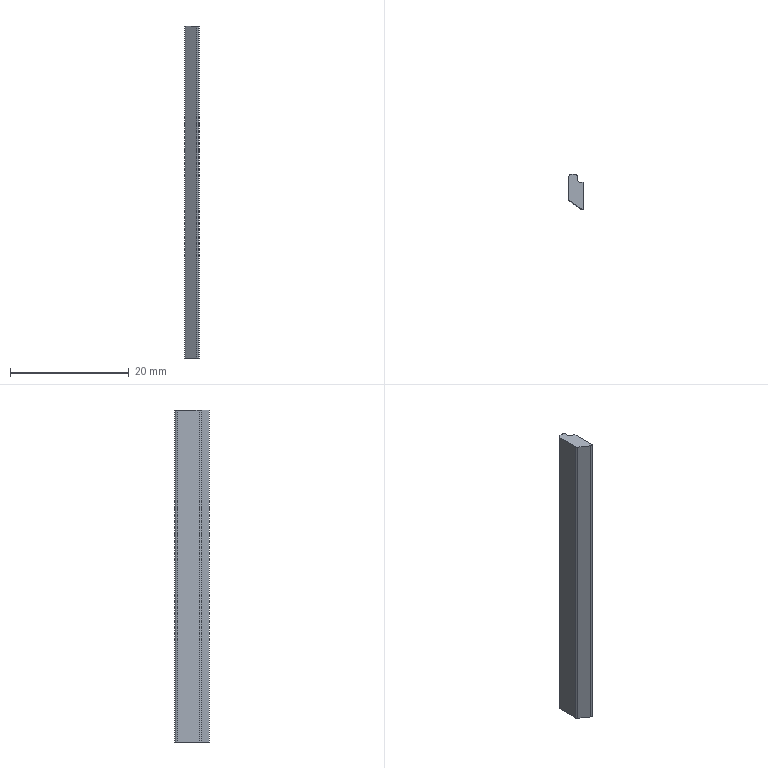Part | NX | features BREP 2 | 2 solids | 28 faces | box 2.447 x 5.891 x 56 mm | volume 1283 mm3 | plane 18 | cylinder 10 | commonest cylinder face diameters 1 x10
STEP:
#1=CARTESIAN_POINT('',(1.064,-2.946,-4.));
#2=VERTEX_POINT('',#1);
#3=CARTESIAN_POINT('',(1.064,-2.946,52.));
#4=VERTEX_POINT('',#3);
#5=CARTESIAN_POINT('',(1.064,-2.946,0.));
#6=DIRECTION('',(0.,0.,1.));
#7=VECTOR('',#6,1000.);
#8=LINE('',#5,#7);
#9=EDGE_CURVE('',#2,#4,#8,.T.);
#10=ORIENTED_EDGE('',*,*,#9,.T.);
#11=CARTESIAN_POINT('',(0.777,-2.855,52.));
#12=VERTEX_POINT('',#11);
#13=CARTESIAN_POINT('',(1.064,-2.446,52.));
#14=DIRECTION('',(0.,0.,1.));
#15=DIRECTION('',(1.,0.,0.));
#16=AXIS2_PLACEMENT_3D('',#13,#14,#15);
#17=CIRCLE('',#16,0.5);
#18=EDGE_CURVE('',#12,#4,#17,.T.);
#19=ORIENTED_EDGE('',*,*,#18,.F.);
#20=CARTESIAN_POINT('',(0.777,-2.855,-4.));
#21=VERTEX_POINT('',#20);
#22=CARTESIAN_POINT('',(0.777,-2.855,0.));
#23=DIRECTION('',(0.,0.,1.));
#24=VECTOR('',#23,1000.);
#25=LINE('',#22,#24);
#26=EDGE_CURVE('',#21,#12,#25,.T.);
#27=ORIENTED_EDGE('',*,*,#26,.F.);
#28=CARTESIAN_POINT('',(1.064,-2.446,-4.));
#29=DIRECTION('',(0.,0.,1.));
#30=DIRECTION('',(1.,0.,0.));
#31=AXIS2_PLACEMENT_3D('',#28,#29,#30);
#32=CIRCLE('',#31,0.5);
#33=EDGE_CURVE('',#21,#2,#32,.T.);
#34=ORIENTED_EDGE('',*,*,#33,.T.);
#35=EDGE_LOOP('',(#10,#19,#27,#34));
#36=FACE_BOUND('',#35,.T.);
#37=CARTESIAN_POINT('',(1.064,-2.446,0.));
#38=DIRECTION('',(0.,0.,1.));
#39=DIRECTION('',(-1.,0.,0.));
#40=AXIS2_PLACEMENT_3D('',#37,#38,#39);
#41=CYLINDRICAL_SURFACE('',#40,0.5);
#42=ADVANCED_FACE('',(#36),#41,.T.);
#43=ORIENTED_EDGE('',*,*,#26,.T.);
#44=CARTESIAN_POINT('',(-1.01,-1.604,52.));
#45=VERTEX_POINT('',#44);
#46=CARTESIAN_POINT('',(0.777,-2.855,52.));
#47=DIRECTION('',(0.8192,-0.5736,0.));
#48=VECTOR('',#47,1000.);
#49=LINE('',#46,#48);
#50=EDGE_CURVE('',#45,#12,#49,.T.);
#51=ORIENTED_EDGE('',*,*,#50,.F.);
#52=CARTESIAN_POINT('',(-1.01,-1.604,-4.));
#53=VERTEX_POINT('',#52);
#54=CARTESIAN_POINT('',(-1.01,-1.604,0.));
#55=DIRECTION('',(0.,0.,1.));
#56=VECTOR('',#55,1000.);
#57=LINE('',#54,#56);
#58=EDGE_CURVE('',#53,#45,#57,.T.);
#59=ORIENTED_EDGE('',*,*,#58,.F.);
#60=CARTESIAN_POINT('',(0.777,-2.855,-4.));
#61=DIRECTION('',(0.8192,-0.5736,0.));
#62=VECTOR('',#61,1000.);
#63=LINE('',#60,#62);
#64=EDGE_CURVE('',#53,#21,#63,.T.);
#65=ORIENTED_EDGE('',*,*,#64,.T.);
#66=EDGE_LOOP('',(#43,#51,#59,#65));
#67=FACE_BOUND('',#66,.T.);
#68=CARTESIAN_POINT('',(0.777,-2.855,0.));
#69=DIRECTION('',(0.5736,0.8192,0.));
#70=DIRECTION('',(0.8192,-0.5736,0.));
#71=AXIS2_PLACEMENT_3D('',#68,#69,#70);
#72=PLANE('',#71);
#73=ADVANCED_FACE('',(#67),#72,.F.);
#74=ORIENTED_EDGE('',*,*,#58,.T.);
#75=CARTESIAN_POINT('',(-1.224,-1.194,52.));
#76=VERTEX_POINT('',#75);
#77=CARTESIAN_POINT('',(-0.7237,-1.194,52.));
#78=DIRECTION('',(0.,0.,1.));
#79=DIRECTION('',(1.,0.,0.));
#80=AXIS2_PLACEMENT_3D('',#77,#78,#79);
#81=CIRCLE('',#80,0.5);
#82=EDGE_CURVE('',#76,#45,#81,.T.);
#83=ORIENTED_EDGE('',*,*,#82,.F.);
#84=CARTESIAN_POINT('',(-1.224,-1.194,-4.));
#85=VERTEX_POINT('',#84);
#86=CARTESIAN_POINT('',(-1.224,-1.194,0.));
#87=DIRECTION('',(0.,0.,1.));
#88=VECTOR('',#87,1000.);
#89=LINE('',#86,#88);
#90=EDGE_CURVE('',#85,#76,#89,.T.);
#91=ORIENTED_EDGE('',*,*,#90,.F.);
#92=CARTESIAN_POINT('',(-0.7237,-1.194,-4.));
#93=DIRECTION('',(0.,0.,1.));
#94=DIRECTION('',(1.,0.,0.));
#95=AXIS2_PLACEMENT_3D('',#92,#93,#94);
#96=CIRCLE('',#95,0.5);
#97=EDGE_CURVE('',#85,#53,#96,.T.);
#98=ORIENTED_EDGE('',*,*,#97,.T.);
#99=EDGE_LOOP('',(#74,#83,#91,#98));
#100=FACE_BOUND('',#99,.T.);
#101=CARTESIAN_POINT('',(-0.7237,-1.194,0.));
#102=DIRECTION('',(0.,0.,1.));
#103=DIRECTION('',(-1.,0.,0.));
#104=AXIS2_PLACEMENT_3D('',#101,#102,#103);
#105=CYLINDRICAL_SURFACE('',#104,0.5);
#106=ADVANCED_FACE('',(#100),#105,.T.);
#107=ORIENTED_EDGE('',*,*,#90,.T.);
#108=CARTESIAN_POINT('',(-1.224,2.446,52.));
#109=VERTEX_POINT('',#108);
#110=CARTESIAN_POINT('',(-1.224,14.446,52.));
#111=DIRECTION('',(0.,-1.,0.));
#112=VECTOR('',#111,1000.);
#113=LINE('',#110,#112);
#114=EDGE_CURVE('',#109,#76,#113,.T.);
#115=ORIENTED_EDGE('',*,*,#114,.F.);
#116=CARTESIAN_POINT('',(-1.224,2.446,-4.));
#117=VERTEX_POINT('',#116);
#118=CARTESIAN_POINT('',(-1.224,2.446,0.));
#119=DIRECTION('',(0.,0.,1.));
#120=VECTOR('',#119,1000.);
#121=LINE('',#118,#120);
#122=EDGE_CURVE('',#117,#109,#121,.T.);
#123=ORIENTED_EDGE('',*,*,#122,.F.);
#124=CARTESIAN_POINT('',(-1.224,14.446,-4.));
#125=DIRECTION('',(0.,-1.,0.));
#126=VECTOR('',#125,1000.);
#127=LINE('',#124,#126);
#128=EDGE_CURVE('',#117,#85,#127,.T.);
#129=ORIENTED_EDGE('',*,*,#128,.T.);
#130=EDGE_LOOP('',(#107,#115,#123,#129));
#131=FACE_BOUND('',#130,.T.);
#132=CARTESIAN_POINT('',(-1.224,-1.194,0.));
#133=DIRECTION('',(1.,0.,0.));
#134=DIRECTION('',(0.,-1.,0.));
#135=AXIS2_PLACEMENT_3D('',#132,#133,#134);
#136=PLANE('',#135);
#137=ADVANCED_FACE('',(#131),#136,.F.);
#138=ORIENTED_EDGE('',*,*,#122,.T.);
#139=CARTESIAN_POINT('',(-0.7237,2.946,52.));
#140=VERTEX_POINT('',#139);
#141=CARTESIAN_POINT('',(-0.7237,2.446,52.));
#142=DIRECTION('',(0.,0.,1.));
#143=DIRECTION('',(1.,0.,0.));
#144=AXIS2_PLACEMENT_3D('',#141,#142,#143);
#145=CIRCLE('',#144,0.5);
#146=EDGE_CURVE('',#140,#109,#145,.T.);
#147=ORIENTED_EDGE('',*,*,#146,.F.);
#148=CARTESIAN_POINT('',(-0.7237,2.946,-4.));
#149=VERTEX_POINT('',#148);
#150=CARTESIAN_POINT('',(-0.7237,2.946,0.));
#151=DIRECTION('',(0.,0.,1.));
#152=VECTOR('',#151,1000.);
#153=LINE('',#150,#152);
#154=EDGE_CURVE('',#149,#140,#153,.T.);
#155=ORIENTED_EDGE('',*,*,#154,.F.);
#156=CARTESIAN_POINT('',(-0.7237,2.446,-4.));
#157=DIRECTION('',(0.,0.,1.));
#158=DIRECTION('',(1.,0.,0.));
#159=AXIS2_PLACEMENT_3D('',#156,#157,#158);
#160=CIRCLE('',#159,0.5);
#161=EDGE_CURVE('',#149,#117,#160,.T.);
#162=ORIENTED_EDGE('',*,*,#161,.T.);
#163=EDGE_LOOP('',(#138,#147,#155,#162));
#164=FACE_BOUND('',#163,.T.);
#165=CARTESIAN_POINT('',(-0.7237,2.446,0.));
#166=DIRECTION('',(0.,0.,1.));
#167=DIRECTION('',(-1.,0.,0.));
#168=AXIS2_PLACEMENT_3D('',#165,#166,#167);
#169=CYLINDRICAL_SURFACE('',#168,0.5);
#170=ADVANCED_FACE('',(#164),#169,.T.);
#171=ORIENTED_EDGE('',*,*,#154,.T.);
#172=CARTESIAN_POINT('',(-0.2237,2.946,52.));
#173=VERTEX_POINT('',#172);
#174=CARTESIAN_POINT('',(-1.25,2.946,52.));
#175=DIRECTION('',(-1.,0.,0.));
#176=VECTOR('',#175,1000.);
#177=LINE('',#174,#176);
#178=EDGE_CURVE('',#173,#140,#177,.T.);
#179=ORIENTED_EDGE('',*,*,#178,.F.);
#180=CARTESIAN_POINT('',(-0.2237,2.946,-4.));
#181=VERTEX_POINT('',#180);
#182=CARTESIAN_POINT('',(-0.2237,2.946,0.));
#183=DIRECTION('',(0.,0.,1.));
#184=VECTOR('',#183,1000.);
#185=LINE('',#182,#184);
#186=EDGE_CURVE('',#181,#173,#185,.T.);
#187=ORIENTED_EDGE('',*,*,#186,.F.);
#188=CARTESIAN_POINT('',(-1.25,2.946,-4.));
#189=DIRECTION('',(-1.,0.,0.));
#190=VECTOR('',#189,1000.);
#191=LINE('',#188,#190);
#192=EDGE_CURVE('',#181,#149,#191,.T.);
#193=ORIENTED_EDGE('',*,*,#192,.T.);
#194=EDGE_LOOP('',(#171,#179,#187,#193));
#195=FACE_BOUND('',#194,.T.);
#196=CARTESIAN_POINT('',(-0.7237,2.946,0.));
#197=DIRECTION('',(0.,-1.,0.));
#198=DIRECTION('',(-1.,0.,0.));
#199=AXIS2_PLACEMENT_3D('',#196,#197,#198);
#200=PLANE('',#199);
#201=ADVANCED_FACE('',(#195),#200,.F.);
#202=ORIENTED_EDGE('',*,*,#186,.T.);
#203=CARTESIAN_POINT('',(0.2763,2.446,52.));
#204=VERTEX_POINT('',#203);
#205=CARTESIAN_POINT('',(-0.2237,2.446,52.));
#206=DIRECTION('',(0.,0.,1.));
#207=DIRECTION('',(1.,0.,0.));
#208=AXIS2_PLACEMENT_3D('',#205,#206,#207);
#209=CIRCLE('',#208,0.5);
#210=EDGE_CURVE('',#204,#173,#209,.T.);
#211=ORIENTED_EDGE('',*,*,#210,.F.);
#212=CARTESIAN_POINT('',(0.2763,2.446,-4.));
#213=VERTEX_POINT('',#212);
#214=CARTESIAN_POINT('',(0.2763,2.446,0.));
#215=DIRECTION('',(0.,0.,1.));
#216=VECTOR('',#215,1000.);
#217=LINE('',#214,#216);
#218=EDGE_CURVE('',#213,#204,#217,.T.);
#219=ORIENTED_EDGE('',*,*,#218,.F.);
#220=CARTESIAN_POINT('',(-0.2237,2.446,-4.));
#221=DIRECTION('',(0.,0.,1.));
#222=DIRECTION('',(1.,0.,0.));
#223=AXIS2_PLACEMENT_3D('',#220,#221,#222);
#224=CIRCLE('',#223,0.5);
#225=EDGE_CURVE('',#213,#181,#224,.T.);
#226=ORIENTED_EDGE('',*,*,#225,.T.);
#227=EDGE_LOOP('',(#202,#211,#219,#226));
#228=FACE_BOUND('',#227,.T.);
#229=CARTESIAN_POINT('',(-0.2237,2.446,0.));
#230=DIRECTION('',(0.,0.,1.));
#231=DIRECTION('',(-1.,0.,0.));
#232=AXIS2_PLACEMENT_3D('',#229,#230,#231);
#233=CYLINDRICAL_SURFACE('',#232,0.5);
#234=ADVANCED_FACE('',(#228),#233,.T.);
#235=ORIENTED_EDGE('',*,*,#218,.T.);
#236=CARTESIAN_POINT('',(0.2763,2.065,52.));
#237=VERTEX_POINT('',#236);
#238=CARTESIAN_POINT('',(0.2763,14.446,52.));
#239=DIRECTION('',(0.,1.,0.));
#240=VECTOR('',#239,1000.);
#241=LINE('',#238,#240);
#242=EDGE_CURVE('',#237,#204,#241,.T.);
#243=ORIENTED_EDGE('',*,*,#242,.F.);
#244=CARTESIAN_POINT('',(0.2763,2.065,-4.));
#245=VERTEX_POINT('',#244);
#246=CARTESIAN_POINT('',(0.2763,2.065,0.));
#247=DIRECTION('',(0.,0.,1.));
#248=VECTOR('',#247,1000.);
#249=LINE('',#246,#248);
#250=EDGE_CURVE('',#245,#237,#249,.T.);
#251=ORIENTED_EDGE('',*,*,#250,.F.);
#252=CARTESIAN_POINT('',(0.2763,14.446,-4.));
#253=DIRECTION('',(0.,1.,0.));
#254=VECTOR('',#253,1000.);
#255=LINE('',#252,#254);
#256=EDGE_CURVE('',#245,#213,#255,.T.);
#257=ORIENTED_EDGE('',*,*,#256,.T.);
#258=EDGE_LOOP('',(#235,#243,#251,#257));
#259=FACE_BOUND('',#258,.T.);
#260=CARTESIAN_POINT('',(0.2763,2.446,0.));
#261=DIRECTION('',(-1.,0.,0.));
#262=DIRECTION('',(0.,1.,0.));
#263=AXIS2_PLACEMENT_3D('',#260,#261,#262);
#264=PLANE('',#263);
#265=ADVANCED_FACE('',(#259),#264,.F.);
#266=ORIENTED_EDGE('',*,*,#250,.T.);
#267=CARTESIAN_POINT('',(0.7763,1.565,52.));
#268=VERTEX_POINT('',#267);
#269=CARTESIAN_POINT('',(0.7763,2.065,52.));
#270=DIRECTION('',(0.,0.,-1.));
#271=DIRECTION('',(1.,0.,0.));
#272=AXIS2_PLACEMENT_3D('',#269,#270,#271);
#273=CIRCLE('',#272,0.5);
#274=EDGE_CURVE('',#268,#237,#273,.T.);
#275=ORIENTED_EDGE('',*,*,#274,.F.);
#276=CARTESIAN_POINT('',(0.7763,1.565,-4.));
#277=VERTEX_POINT('',#276);
#278=CARTESIAN_POINT('',(0.7763,1.565,0.));
#279=DIRECTION('',(0.,0.,1.));
#280=VECTOR('',#279,1000.);
#281=LINE('',#278,#280);
#282=EDGE_CURVE('',#277,#268,#281,.T.);
#283=ORIENTED_EDGE('',*,*,#282,.F.);
#284=CARTESIAN_POINT('',(0.7763,2.065,-4.));
#285=DIRECTION('',(0.,0.,-1.));
#286=DIRECTION('',(1.,0.,0.));
#287=AXIS2_PLACEMENT_3D('',#284,#285,#286);
#288=CIRCLE('',#287,0.5);
#289=EDGE_CURVE('',#277,#245,#288,.T.);
#290=ORIENTED_EDGE('',*,*,#289,.T.);
#291=EDGE_LOOP('',(#266,#275,#283,#290));
#292=FACE_BOUND('',#291,.T.);
#293=CARTESIAN_POINT('',(0.7763,2.065,0.));
#294=DIRECTION('',(0.,0.,1.));
#295=DIRECTION('',(-1.,0.,0.));
#296=AXIS2_PLACEMENT_3D('',#293,#294,#295);
#297=CYLINDRICAL_SURFACE('',#296,0.5);
#298=ADVANCED_FACE('',(#292),#297,.F.);
#299=ORIENTED_EDGE('',*,*,#282,.T.);
#300=CARTESIAN_POINT('',(1.224,1.565,52.));
#301=VERTEX_POINT('',#300);
#302=CARTESIAN_POINT('',(-1.25,1.565,52.));
#303=DIRECTION('',(-1.,0.,0.));
#304=VECTOR('',#303,1000.);
#305=LINE('',#302,#304);
#306=EDGE_CURVE('',#301,#268,#305,.T.);
#307=ORIENTED_EDGE('',*,*,#306,.F.);
#308=CARTESIAN_POINT('',(1.224,1.565,-4.));
#309=VERTEX_POINT('',#308);
#310=CARTESIAN_POINT('',(1.224,1.565,0.));
#311=DIRECTION('',(0.,0.,1.));
#312=VECTOR('',#311,1000.);
#313=LINE('',#310,#312);
#314=EDGE_CURVE('',#309,#301,#313,.T.);
#315=ORIENTED_EDGE('',*,*,#314,.F.);
#316=CARTESIAN_POINT('',(-1.25,1.565,-4.));
#317=DIRECTION('',(-1.,0.,0.));
#318=VECTOR('',#317,1000.);
#319=LINE('',#316,#318);
#320=EDGE_CURVE('',#309,#277,#319,.T.);
#321=ORIENTED_EDGE('',*,*,#320,.T.);
#322=EDGE_LOOP('',(#299,#307,#315,#321));
#323=FACE_BOUND('',#322,.T.);
#324=CARTESIAN_POINT('',(0.7763,1.565,0.));
#325=DIRECTION('',(0.,-1.,0.));
#326=DIRECTION('',(-1.,0.,0.));
#327=AXIS2_PLACEMENT_3D('',#324,#325,#326);
#328=PLANE('',#327);
#329=ADVANCED_FACE('',(#323),#328,.F.);
#330=ORIENTED_EDGE('',*,*,#314,.T.);
#331=CARTESIAN_POINT('',(1.224,-2.946,52.));
#332=VERTEX_POINT('',#331);
#333=CARTESIAN_POINT('',(1.224,14.446,52.));
#334=DIRECTION('',(0.,1.,0.));
#335=VECTOR('',#334,1000.);
#336=LINE('',#333,#335);
#337=EDGE_CURVE('',#332,#301,#336,.T.);
#338=ORIENTED_EDGE('',*,*,#337,.F.);
#339=CARTESIAN_POINT('',(1.224,-2.946,-4.));
#340=VERTEX_POINT('',#339);
#341=CARTESIAN_POINT('',(1.224,-2.946,0.));
#342=DIRECTION('',(0.,0.,1.));
#343=VECTOR('',#342,1000.);
#344=LINE('',#341,#343);
#345=EDGE_CURVE('',#340,#332,#344,.T.);
#346=ORIENTED_EDGE('',*,*,#345,.F.);
#347=CARTESIAN_POINT('',(1.224,14.446,-4.));
#348=DIRECTION('',(0.,1.,0.));
#349=VECTOR('',#348,1000.);
#350=LINE('',#347,#349);
#351=EDGE_CURVE('',#340,#309,#350,.T.);
#352=ORIENTED_EDGE('',*,*,#351,.T.);
#353=EDGE_LOOP('',(#330,#338,#346,#352));
#354=FACE_BOUND('',#353,.T.);
#355=CARTESIAN_POINT('',(1.224,14.446,0.));
#356=DIRECTION('',(-1.,0.,0.));
#357=DIRECTION('',(0.,1.,0.));
#358=AXIS2_PLACEMENT_3D('',#355,#356,#357);
#359=PLANE('',#358);
#360=ADVANCED_FACE('',(#354),#359,.F.);
#361=CARTESIAN_POINT('',(-1.25,-2.946,-4.));
#362=DIRECTION('',(1.,0.,0.));
#363=VECTOR('',#362,1000.);
#364=LINE('',#361,#363);
#365=EDGE_CURVE('',#2,#340,#364,.T.);
#366=ORIENTED_EDGE('',*,*,#365,.T.);
#367=ORIENTED_EDGE('',*,*,#345,.T.);
#368=CARTESIAN_POINT('',(-1.25,-2.946,52.));
#369=DIRECTION('',(1.,0.,0.));
#370=VECTOR('',#369,1000.);
#371=LINE('',#368,#370);
#372=EDGE_CURVE('',#4,#332,#371,.T.);
#373=ORIENTED_EDGE('',*,*,#372,.F.);
#374=ORIENTED_EDGE('',*,*,#9,.F.);
#375=EDGE_LOOP('',(#366,#367,#373,#374));
#376=FACE_BOUND('',#375,.T.);
#377=CARTESIAN_POINT('',(2.488,-2.946,0.));
#378=DIRECTION('',(0.,1.,0.));
#379=DIRECTION('',(1.,0.,0.));
#380=AXIS2_PLACEMENT_3D('',#377,#378,#379);
#381=PLANE('',#380);
#382=ADVANCED_FACE('',(#376),#381,.F.);
#383=ORIENTED_EDGE('',*,*,#337,.T.);
#384=ORIENTED_EDGE('',*,*,#306,.T.);
#385=ORIENTED_EDGE('',*,*,#274,.T.);
#386=ORIENTED_EDGE('',*,*,#242,.T.);
#387=ORIENTED_EDGE('',*,*,#210,.T.);
#388=ORIENTED_EDGE('',*,*,#178,.T.);
#389=ORIENTED_EDGE('',*,*,#146,.T.);
#390=ORIENTED_EDGE('',*,*,#114,.T.);
#391=ORIENTED_EDGE('',*,*,#82,.T.);
#392=ORIENTED_EDGE('',*,*,#50,.T.);
#393=ORIENTED_EDGE('',*,*,#18,.T.);
#394=ORIENTED_EDGE('',*,*,#372,.T.);
#395=EDGE_LOOP('',(#383,#384,#385,#386,#387,#388,#389,#390,#391,#392,#393,#394));
#396=FACE_BOUND('',#395,.T.);
#397=CARTESIAN_POINT('',(-1.25,14.446,52.));
#398=DIRECTION('',(0.,0.,1.));
#399=DIRECTION('',(-1.,0.,0.));
#400=AXIS2_PLACEMENT_3D('',#397,#398,#399);
#401=PLANE('',#400);
#402=ADVANCED_FACE('',(#396),#401,.T.);
#403=ORIENTED_EDGE('',*,*,#351,.F.);
#404=ORIENTED_EDGE('',*,*,#365,.F.);
#405=ORIENTED_EDGE('',*,*,#33,.F.);
#406=ORIENTED_EDGE('',*,*,#64,.F.);
#407=ORIENTED_EDGE('',*,*,#97,.F.);
#408=ORIENTED_EDGE('',*,*,#128,.F.);
#409=ORIENTED_EDGE('',*,*,#161,.F.);
#410=ORIENTED_EDGE('',*,*,#192,.F.);
#411=ORIENTED_EDGE('',*,*,#225,.F.);
#412=ORIENTED_EDGE('',*,*,#256,.F.);
#413=ORIENTED_EDGE('',*,*,#289,.F.);
#414=ORIENTED_EDGE('',*,*,#320,.F.);
#415=EDGE_LOOP('',(#403,#404,#405,#406,#407,#408,#409,#410,#411,#412,#413,#414));
#416=FACE_BOUND('',#415,.T.);
#417=CARTESIAN_POINT('',(-1.25,14.446,-4.));
#418=DIRECTION('',(0.,0.,1.));
#419=DIRECTION('',(-1.,0.,0.));
#420=AXIS2_PLACEMENT_3D('',#417,#418,#419);
#421=PLANE('',#420);
#422=ADVANCED_FACE('',(#416),#421,.F.);
#423=CLOSED_SHELL('',(#42,#73,#106,#137,#170,#201,#234,#265,#298,#329,#360,#382,#402,#422));
#424=MANIFOLD_SOLID_BREP('',#423);
#425=CARTESIAN_POINT('',(1.064,-2.946,-4.));
#426=VERTEX_POINT('',#425);
#427=CARTESIAN_POINT('',(1.064,-2.946,52.));
#428=VERTEX_POINT('',#427);
#429=CARTESIAN_POINT('',(1.064,-2.946,0.));
#430=DIRECTION('',(0.,0.,1.));
#431=VECTOR('',#430,1000.);
#432=LINE('',#429,#431);
#433=EDGE_CURVE('',#426,#428,#432,.T.);
#434=ORIENTED_EDGE('',*,*,#433,.T.);
#435=CARTESIAN_POINT('',(0.777,-2.855,52.));
#436=VERTEX_POINT('',#435);
#437=CARTESIAN_POINT('',(1.064,-2.446,52.));
#438=DIRECTION('',(0.,0.,1.));
#439=DIRECTION('',(1.,0.,0.));
#440=AXIS2_PLACEMENT_3D('',#437,#438,#439);
#441=CIRCLE('',#440,0.5);
#442=EDGE_CURVE('',#436,#428,#441,.T.);
#443=ORIENTED_EDGE('',*,*,#442,.F.);
#444=CARTESIAN_POINT('',(0.777,-2.855,-4.));
#445=VERTEX_POINT('',#444);
#446=CARTESIAN_POINT('',(0.777,-2.855,0.));
#447=DIRECTION('',(0.,0.,1.));
#448=VECTOR('',#447,1000.);
#449=LINE('',#446,#448);
#450=EDGE_CURVE('',#445,#436,#449,.T.);
#451=ORIENTED_EDGE('',*,*,#450,.F.);
#452=CARTESIAN_POINT('',(1.064,-2.446,-4.));
#453=DIRECTION('',(0.,0.,1.));
#454=DIRECTION('',(1.,0.,0.));
#455=AXIS2_PLACEMENT_3D('',#452,#453,#454);
#456=CIRCLE('',#455,0.5);
#457=EDGE_CURVE('',#445,#426,#456,.T.);
#458=ORIENTED_EDGE('',*,*,#457,.T.);
#459=EDGE_LOOP('',(#434,#443,#451,#458));
#460=FACE_BOUND('',#459,.T.);
#461=CARTESIAN_POINT('',(1.064,-2.446,0.));
#462=DIRECTION('',(0.,0.,1.));
#463=DIRECTION('',(-1.,0.,0.));
#464=AXIS2_PLACEMENT_3D('',#461,#462,#463);
#465=CYLINDRICAL_SURFACE('',#464,0.5);
#466=ADVANCED_FACE('',(#460),#465,.T.);
#467=ORIENTED_EDGE('',*,*,#450,.T.);
#468=CARTESIAN_POINT('',(-1.01,-1.604,52.));
#469=VERTEX_POINT('',#468);
#470=CARTESIAN_POINT('',(0.777,-2.855,52.));
#471=DIRECTION('',(0.8192,-0.5736,0.));
#472=VECTOR('',#471,1000.);
#473=LINE('',#470,#472);
#474=EDGE_CURVE('',#469,#436,#473,.T.);
#475=ORIENTED_EDGE('',*,*,#474,.F.);
#476=CARTESIAN_POINT('',(-1.01,-1.604,-4.));
#477=VERTEX_POINT('',#476);
#478=CARTESIAN_POINT('',(-1.01,-1.604,0.));
#479=DIRECTION('',(0.,0.,1.));
#480=VECTOR('',#479,1000.);
#481=LINE('',#478,#480);
#482=EDGE_CURVE('',#477,#469,#481,.T.);
#483=ORIENTED_EDGE('',*,*,#482,.F.);
#484=CARTESIAN_POINT('',(0.777,-2.855,-4.));
#485=DIRECTION('',(0.8192,-0.5736,0.));
#486=VECTOR('',#485,1000.);
#487=LINE('',#484,#486);
#488=EDGE_CURVE('',#477,#445,#487,.T.);
#489=ORIENTED_EDGE('',*,*,#488,.T.);
#490=EDGE_LOOP('',(#467,#475,#483,#489));
#491=FACE_BOUND('',#490,.T.);
#492=CARTESIAN_POINT('',(0.777,-2.855,0.));
#493=DIRECTION('',(0.5736,0.8192,0.));
#494=DIRECTION('',(0.8192,-0.5736,0.));
#495=AXIS2_PLACEMENT_3D('',#492,#493,#494);
#496=PLANE('',#495);
#497=ADVANCED_FACE('',(#491),#496,.F.);
#498=ORIENTED_EDGE('',*,*,#482,.T.);
#499=CARTESIAN_POINT('',(-1.224,-1.194,52.));
#500=VERTEX_POINT('',#499);
#501=CARTESIAN_POINT('',(-0.7237,-1.194,52.));
#502=DIRECTION('',(0.,0.,1.));
#503=DIRECTION('',(1.,0.,0.));
#504=AXIS2_PLACEMENT_3D('',#501,#502,#503);
#505=CIRCLE('',#504,0.5);
#506=EDGE_CURVE('',#500,#469,#505,.T.);
#507=ORIENTED_EDGE('',*,*,#506,.F.);
#508=CARTESIAN_POINT('',(-1.224,-1.194,-4.));
#509=VERTEX_POINT('',#508);
#510=CARTESIAN_POINT('',(-1.224,-1.194,0.));
#511=DIRECTION('',(0.,0.,1.));
#512=VECTOR('',#511,1000.);
#513=LINE('',#510,#512);
#514=EDGE_CURVE('',#509,#500,#513,.T.);
#515=ORIENTED_EDGE('',*,*,#514,.F.);
#516=CARTESIAN_POINT('',(-0.7237,-1.194,-4.));
#517=DIRECTION('',(0.,0.,1.));
#518=DIRECTION('',(1.,0.,0.));
#519=AXIS2_PLACEMENT_3D('',#516,#517,#518);
#520=CIRCLE('',#519,0.5);
#521=EDGE_CURVE('',#509,#477,#520,.T.);
#522=ORIENTED_EDGE('',*,*,#521,.T.);
#523=EDGE_LOOP('',(#498,#507,#515,#522));
#524=FACE_BOUND('',#523,.T.);
#525=CARTESIAN_POINT('',(-0.7237,-1.194,0.));
#526=DIRECTION('',(0.,0.,1.));
#527=DIRECTION('',(-1.,0.,0.));
#528=AXIS2_PLACEMENT_3D('',#525,#526,#527);
#529=CYLINDRICAL_SURFACE('',#528,0.5);
#530=ADVANCED_FACE('',(#524),#529,.T.);
#531=ORIENTED_EDGE('',*,*,#514,.T.);
#532=CARTESIAN_POINT('',(-1.224,2.446,52.));
#533=VERTEX_POINT('',#532);
#534=CARTESIAN_POINT('',(-1.224,14.446,52.));
#535=DIRECTION('',(0.,-1.,0.));
#536=VECTOR('',#535,1000.);
#537=LINE('',#534,#536);
#538=EDGE_CURVE('',#533,#500,#537,.T.);
#539=ORIENTED_EDGE('',*,*,#538,.F.);
#540=CARTESIAN_POINT('',(-1.224,2.446,-4.));
#541=VERTEX_POINT('',#540);
#542=CARTESIAN_POINT('',(-1.224,2.446,0.));
#543=DIRECTION('',(0.,0.,1.));
#544=VECTOR('',#543,1000.);
#545=LINE('',#542,#544);
#546=EDGE_CURVE('',#541,#533,#545,.T.);
#547=ORIENTED_EDGE('',*,*,#546,.F.);
#548=CARTESIAN_POINT('',(-1.224,14.446,-4.));
#549=DIRECTION('',(0.,-1.,0.));
#550=VECTOR('',#549,1000.);
#551=LINE('',#548,#550);
#552=EDGE_CURVE('',#541,#509,#551,.T.);
#553=ORIENTED_EDGE('',*,*,#552,.T.);
#554=EDGE_LOOP('',(#531,#539,#547,#553));
#555=FACE_BOUND('',#554,.T.);
#556=CARTESIAN_POINT('',(-1.224,-1.194,0.));
#557=DIRECTION('',(1.,0.,0.));
#558=DIRECTION('',(0.,-1.,0.));
#559=AXIS2_PLACEMENT_3D('',#556,#557,#558);
#560=PLANE('',#559);
#561=ADVANCED_FACE('',(#555),#560,.F.);
#562=ORIENTED_EDGE('',*,*,#546,.T.);
#563=CARTESIAN_POINT('',(-0.7237,2.946,52.));
#564=VERTEX_POINT('',#563);
#565=CARTESIAN_POINT('',(-0.7237,2.446,52.));
#566=DIRECTION('',(0.,0.,1.));
#567=DIRECTION('',(1.,0.,0.));
#568=AXIS2_PLACEMENT_3D('',#565,#566,#567);
#569=CIRCLE('',#568,0.5);
#570=EDGE_CURVE('',#564,#533,#569,.T.);
#571=ORIENTED_EDGE('',*,*,#570,.F.);
#572=CARTESIAN_POINT('',(-0.7237,2.946,-4.));
#573=VERTEX_POINT('',#572);
#574=CARTESIAN_POINT('',(-0.7237,2.946,0.));
#575=DIRECTION('',(0.,0.,1.));
#576=VECTOR('',#575,1000.);
#577=LINE('',#574,#576);
#578=EDGE_CURVE('',#573,#564,#577,.T.);
#579=ORIENTED_EDGE('',*,*,#578,.F.);
#580=CARTESIAN_POINT('',(-0.7237,2.446,-4.));
#581=DIRECTION('',(0.,0.,1.));
#582=DIRECTION('',(1.,0.,0.));
#583=AXIS2_PLACEMENT_3D('',#580,#581,#582);
#584=CIRCLE('',#583,0.5);
#585=EDGE_CURVE('',#573,#541,#584,.T.);
#586=ORIENTED_EDGE('',*,*,#585,.T.);
#587=EDGE_LOOP('',(#562,#571,#579,#586));
#588=FACE_BOUND('',#587,.T.);
#589=CARTESIAN_POINT('',(-0.7237,2.446,0.));
#590=DIRECTION('',(0.,0.,1.));
#591=DIRECTION('',(-1.,0.,0.));
#592=AXIS2_PLACEMENT_3D('',#589,#590,#591);
#593=CYLINDRICAL_SURFACE('',#592,0.5);
#594=ADVANCED_FACE('',(#588),#593,.T.);
#595=ORIENTED_EDGE('',*,*,#578,.T.);
#596=CARTESIAN_POINT('',(-0.2237,2.946,52.));
#597=VERTEX_POINT('',#596);
#598=CARTESIAN_POINT('',(-1.25,2.946,52.));
#599=DIRECTION('',(-1.,0.,0.));
#600=VECTOR('',#599,1000.);
#601=LINE('',#598,#600);
#602=EDGE_CURVE('',#597,#564,#601,.T.);
#603=ORIENTED_EDGE('',*,*,#602,.F.);
#604=CARTESIAN_POINT('',(-0.2237,2.946,-4.));
#605=VERTEX_POINT('',#604);
#606=CARTESIAN_POINT('',(-0.2237,2.946,0.));
#607=DIRECTION('',(0.,0.,1.));
#608=VECTOR('',#607,1000.);
#609=LINE('',#606,#608);
#610=EDGE_CURVE('',#605,#597,#609,.T.);
#611=ORIENTED_EDGE('',*,*,#610,.F.);
#612=CARTESIAN_POINT('',(-1.25,2.946,-4.));
#613=DIRECTION('',(-1.,0.,0.));
#614=VECTOR('',#613,1000.);
#615=LINE('',#612,#614);
#616=EDGE_CURVE('',#605,#573,#615,.T.);
#617=ORIENTED_EDGE('',*,*,#616,.T.);
#618=EDGE_LOOP('',(#595,#603,#611,#617));
#619=FACE_BOUND('',#618,.T.);
#620=CARTESIAN_POINT('',(-0.7237,2.946,0.));
#621=DIRECTION('',(0.,-1.,0.));
#622=DIRECTION('',(-1.,0.,0.));
#623=AXIS2_PLACEMENT_3D('',#620,#621,#622);
#624=PLANE('',#623);
#625=ADVANCED_FACE('',(#619),#624,.F.);
#626=ORIENTED_EDGE('',*,*,#610,.T.);
#627=CARTESIAN_POINT('',(0.2763,2.446,52.));
#628=VERTEX_POINT('',#627);
#629=CARTESIAN_POINT('',(-0.2237,2.446,52.));
#630=DIRECTION('',(0.,0.,1.));
#631=DIRECTION('',(1.,0.,0.));
#632=AXIS2_PLACEMENT_3D('',#629,#630,#631);
#633=CIRCLE('',#632,0.5);
#634=EDGE_CURVE('',#628,#597,#633,.T.);
#635=ORIENTED_EDGE('',*,*,#634,.F.);
#636=CARTESIAN_POINT('',(0.2763,2.446,-4.));
#637=VERTEX_POINT('',#636);
#638=CARTESIAN_POINT('',(0.2763,2.446,0.));
#639=DIRECTION('',(0.,0.,1.));
#640=VECTOR('',#639,1000.);
#641=LINE('',#638,#640);
#642=EDGE_CURVE('',#637,#628,#641,.T.);
#643=ORIENTED_EDGE('',*,*,#642,.F.);
#644=CARTESIAN_POINT('',(-0.2237,2.446,-4.));
#645=DIRECTION('',(0.,0.,1.));
#646=DIRECTION('',(1.,0.,0.));
#647=AXIS2_PLACEMENT_3D('',#644,#645,#646);
#648=CIRCLE('',#647,0.5);
#649=EDGE_CURVE('',#637,#605,#648,.T.);
#650=ORIENTED_EDGE('',*,*,#649,.T.);
#651=EDGE_LOOP('',(#626,#635,#643,#650));
#652=FACE_BOUND('',#651,.T.);
#653=CARTESIAN_POINT('',(-0.2237,2.446,0.));
#654=DIRECTION('',(0.,0.,1.));
#655=DIRECTION('',(-1.,0.,0.));
#656=AXIS2_PLACEMENT_3D('',#653,#654,#655);
#657=CYLINDRICAL_SURFACE('',#656,0.5);
#658=ADVANCED_FACE('',(#652),#657,.T.);
#659=ORIENTED_EDGE('',*,*,#642,.T.);
#660=CARTESIAN_POINT('',(0.2763,2.065,52.));
#661=VERTEX_POINT('',#660);
#662=CARTESIAN_POINT('',(0.2763,14.446,52.));
#663=DIRECTION('',(0.,1.,0.));
#664=VECTOR('',#663,1000.);
#665=LINE('',#662,#664);
#666=EDGE_CURVE('',#661,#628,#665,.T.);
#667=ORIENTED_EDGE('',*,*,#666,.F.);
#668=CARTESIAN_POINT('',(0.2763,2.065,-4.));
#669=VERTEX_POINT('',#668);
#670=CARTESIAN_POINT('',(0.2763,2.065,0.));
#671=DIRECTION('',(0.,0.,1.));
#672=VECTOR('',#671,1000.);
#673=LINE('',#670,#672);
#674=EDGE_CURVE('',#669,#661,#673,.T.);
#675=ORIENTED_EDGE('',*,*,#674,.F.);
#676=CARTESIAN_POINT('',(0.2763,14.446,-4.));
#677=DIRECTION('',(0.,1.,0.));
#678=VECTOR('',#677,1000.);
#679=LINE('',#676,#678);
#680=EDGE_CURVE('',#669,#637,#679,.T.);
#681=ORIENTED_EDGE('',*,*,#680,.T.);
#682=EDGE_LOOP('',(#659,#667,#675,#681));
#683=FACE_BOUND('',#682,.T.);
#684=CARTESIAN_POINT('',(0.2763,2.446,0.));
#685=DIRECTION('',(-1.,0.,0.));
#686=DIRECTION('',(0.,1.,0.));
#687=AXIS2_PLACEMENT_3D('',#684,#685,#686);
#688=PLANE('',#687);
#689=ADVANCED_FACE('',(#683),#688,.F.);
#690=ORIENTED_EDGE('',*,*,#674,.T.);
#691=CARTESIAN_POINT('',(0.7763,1.565,52.));
#692=VERTEX_POINT('',#691);
#693=CARTESIAN_POINT('',(0.7763,2.065,52.));
#694=DIRECTION('',(0.,0.,-1.));
#695=DIRECTION('',(1.,0.,0.));
#696=AXIS2_PLACEMENT_3D('',#693,#694,#695);
#697=CIRCLE('',#696,0.5);
#698=EDGE_CURVE('',#692,#661,#697,.T.);
#699=ORIENTED_EDGE('',*,*,#698,.F.);
#700=CARTESIAN_POINT('',(0.7763,1.565,-4.));
#701=VERTEX_POINT('',#700);
#702=CARTESIAN_POINT('',(0.7763,1.565,0.));
#703=DIRECTION('',(0.,0.,1.));
#704=VECTOR('',#703,1000.);
#705=LINE('',#702,#704);
#706=EDGE_CURVE('',#701,#692,#705,.T.);
#707=ORIENTED_EDGE('',*,*,#706,.F.);
#708=CARTESIAN_POINT('',(0.7763,2.065,-4.));
#709=DIRECTION('',(0.,0.,-1.));
#710=DIRECTION('',(1.,0.,0.));
#711=AXIS2_PLACEMENT_3D('',#708,#709,#710);
#712=CIRCLE('',#711,0.5);
#713=EDGE_CURVE('',#701,#669,#712,.T.);
#714=ORIENTED_EDGE('',*,*,#713,.T.);
#715=EDGE_LOOP('',(#690,#699,#707,#714));
#716=FACE_BOUND('',#715,.T.);
#717=CARTESIAN_POINT('',(0.7763,2.065,0.));
#718=DIRECTION('',(0.,0.,1.));
#719=DIRECTION('',(-1.,0.,0.));
#720=AXIS2_PLACEMENT_3D('',#717,#718,#719);
#721=CYLINDRICAL_SURFACE('',#720,0.5);
#722=ADVANCED_FACE('',(#716),#721,.F.);
#723=ORIENTED_EDGE('',*,*,#706,.T.);
#724=CARTESIAN_POINT('',(1.224,1.565,52.));
#725=VERTEX_POINT('',#724);
#726=CARTESIAN_POINT('',(-1.25,1.565,52.));
#727=DIRECTION('',(-1.,0.,0.));
#728=VECTOR('',#727,1000.);
#729=LINE('',#726,#728);
#730=EDGE_CURVE('',#725,#692,#729,.T.);
#731=ORIENTED_EDGE('',*,*,#730,.F.);
#732=CARTESIAN_POINT('',(1.224,1.565,-4.));
#733=VERTEX_POINT('',#732);
#734=CARTESIAN_POINT('',(1.224,1.565,0.));
#735=DIRECTION('',(0.,0.,1.));
#736=VECTOR('',#735,1000.);
#737=LINE('',#734,#736);
#738=EDGE_CURVE('',#733,#725,#737,.T.);
#739=ORIENTED_EDGE('',*,*,#738,.F.);
#740=CARTESIAN_POINT('',(-1.25,1.565,-4.));
#741=DIRECTION('',(-1.,0.,0.));
#742=VECTOR('',#741,1000.);
#743=LINE('',#740,#742);
#744=EDGE_CURVE('',#733,#701,#743,.T.);
#745=ORIENTED_EDGE('',*,*,#744,.T.);
#746=EDGE_LOOP('',(#723,#731,#739,#745));
#747=FACE_BOUND('',#746,.T.);
#748=CARTESIAN_POINT('',(0.7763,1.565,0.));
#749=DIRECTION('',(0.,-1.,0.));
#750=DIRECTION('',(-1.,0.,0.));
#751=AXIS2_PLACEMENT_3D('',#748,#749,#750);
#752=PLANE('',#751);
#753=ADVANCED_FACE('',(#747),#752,.F.);
#754=ORIENTED_EDGE('',*,*,#738,.T.);
#755=CARTESIAN_POINT('',(1.224,-2.946,52.));
#756=VERTEX_POINT('',#755);
#757=CARTESIAN_POINT('',(1.224,14.446,52.));
#758=DIRECTION('',(0.,1.,0.));
#759=VECTOR('',#758,1000.);
#760=LINE('',#757,#759);
#761=EDGE_CURVE('',#756,#725,#760,.T.);
#762=ORIENTED_EDGE('',*,*,#761,.F.);
#763=CARTESIAN_POINT('',(1.224,-2.946,-4.));
#764=VERTEX_POINT('',#763);
#765=CARTESIAN_POINT('',(1.224,-2.946,0.));
#766=DIRECTION('',(0.,0.,1.));
#767=VECTOR('',#766,1000.);
#768=LINE('',#765,#767);
#769=EDGE_CURVE('',#764,#756,#768,.T.);
#770=ORIENTED_EDGE('',*,*,#769,.F.);
#771=CARTESIAN_POINT('',(1.224,14.446,-4.));
#772=DIRECTION('',(0.,1.,0.));
#773=VECTOR('',#772,1000.);
#774=LINE('',#771,#773);
#775=EDGE_CURVE('',#764,#733,#774,.T.);
#776=ORIENTED_EDGE('',*,*,#775,.T.);
#777=EDGE_LOOP('',(#754,#762,#770,#776));
#778=FACE_BOUND('',#777,.T.);
#779=CARTESIAN_POINT('',(1.224,14.446,0.));
#780=DIRECTION('',(-1.,0.,0.));
#781=DIRECTION('',(0.,1.,0.));
#782=AXIS2_PLACEMENT_3D('',#779,#780,#781);
#783=PLANE('',#782);
#784=ADVANCED_FACE('',(#778),#783,.F.);
#785=CARTESIAN_POINT('',(-1.25,-2.946,-4.));
#786=DIRECTION('',(1.,0.,0.));
#787=VECTOR('',#786,1000.);
#788=LINE('',#785,#787);
#789=EDGE_CURVE('',#426,#764,#788,.T.);
#790=ORIENTED_EDGE('',*,*,#789,.T.);
#791=ORIENTED_EDGE('',*,*,#769,.T.);
#792=CARTESIAN_POINT('',(-1.25,-2.946,52.));
#793=DIRECTION('',(1.,0.,0.));
#794=VECTOR('',#793,1000.);
#795=LINE('',#792,#794);
#796=EDGE_CURVE('',#428,#756,#795,.T.);
#797=ORIENTED_EDGE('',*,*,#796,.F.);
#798=ORIENTED_EDGE('',*,*,#433,.F.);
#799=EDGE_LOOP('',(#790,#791,#797,#798));
#800=FACE_BOUND('',#799,.T.);
#801=CARTESIAN_POINT('',(2.488,-2.946,0.));
#802=DIRECTION('',(0.,1.,0.));
#803=DIRECTION('',(1.,0.,0.));
#804=AXIS2_PLACEMENT_3D('',#801,#802,#803);
#805=PLANE('',#804);
#806=ADVANCED_FACE('',(#800),#805,.F.);
#807=ORIENTED_EDGE('',*,*,#761,.T.);
#808=ORIENTED_EDGE('',*,*,#730,.T.);
#809=ORIENTED_EDGE('',*,*,#698,.T.);
#810=ORIENTED_EDGE('',*,*,#666,.T.);
#811=ORIENTED_EDGE('',*,*,#634,.T.);
#812=ORIENTED_EDGE('',*,*,#602,.T.);
#813=ORIENTED_EDGE('',*,*,#570,.T.);
#814=ORIENTED_EDGE('',*,*,#538,.T.);
#815=ORIENTED_EDGE('',*,*,#506,.T.);
#816=ORIENTED_EDGE('',*,*,#474,.T.);
#817=ORIENTED_EDGE('',*,*,#442,.T.);
#818=ORIENTED_EDGE('',*,*,#796,.T.);
#819=EDGE_LOOP('',(#807,#808,#809,#810,#811,#812,#813,#814,#815,#816,#817,#818));
#820=FACE_BOUND('',#819,.T.);
#821=CARTESIAN_POINT('',(-1.25,14.446,52.));
#822=DIRECTION('',(0.,0.,1.));
#823=DIRECTION('',(-1.,0.,0.));
#824=AXIS2_PLACEMENT_3D('',#821,#822,#823);
#825=PLANE('',#824);
#826=ADVANCED_FACE('',(#820),#825,.T.);
#827=ORIENTED_EDGE('',*,*,#775,.F.);
#828=ORIENTED_EDGE('',*,*,#789,.F.);
#829=ORIENTED_EDGE('',*,*,#457,.F.);
#830=ORIENTED_EDGE('',*,*,#488,.F.);
#831=ORIENTED_EDGE('',*,*,#521,.F.);
#832=ORIENTED_EDGE('',*,*,#552,.F.);
#833=ORIENTED_EDGE('',*,*,#585,.F.);
#834=ORIENTED_EDGE('',*,*,#616,.F.);
#835=ORIENTED_EDGE('',*,*,#649,.F.);
#836=ORIENTED_EDGE('',*,*,#680,.F.);
#837=ORIENTED_EDGE('',*,*,#713,.F.);
#838=ORIENTED_EDGE('',*,*,#744,.F.);
#839=EDGE_LOOP('',(#827,#828,#829,#830,#831,#832,#833,#834,#835,#836,#837,#838));
#840=FACE_BOUND('',#839,.T.);
#841=CARTESIAN_POINT('',(-1.25,14.446,-4.));
#842=DIRECTION('',(0.,0.,1.));
#843=DIRECTION('',(-1.,0.,0.));
#844=AXIS2_PLACEMENT_3D('',#841,#842,#843);
#845=PLANE('',#844);
#846=ADVANCED_FACE('',(#840),#845,.F.);
#847=CLOSED_SHELL('',(#466,#497,#530,#561,#594,#625,#658,#689,#722,#753,#784,#806,#826,#846));
#848=MANIFOLD_SOLID_BREP('',#847);
#849=(LENGTH_UNIT()NAMED_UNIT(*)SI_UNIT(.MILLI.,.METRE.));
#850=UNCERTAINTY_MEASURE_WITH_UNIT(LENGTH_MEASURE(0.00001),#849,'','');
#851=(NAMED_UNIT(*)PLANE_ANGLE_UNIT()SI_UNIT($,.RADIAN.));
#852=(NAMED_UNIT(*)SI_UNIT($,.STERADIAN.)SOLID_ANGLE_UNIT());
#853=(GEOMETRIC_REPRESENTATION_CONTEXT(3)GLOBAL_UNCERTAINTY_ASSIGNED_CONTEXT((#850))GLOBAL_UNIT_ASSIGNED_CONTEXT((#849,#851,#852))REPRESENTATION_CONTEXT('',''));
#854=ADVANCED_BREP_SHAPE_REPRESENTATION('',(#424,#848),#853);